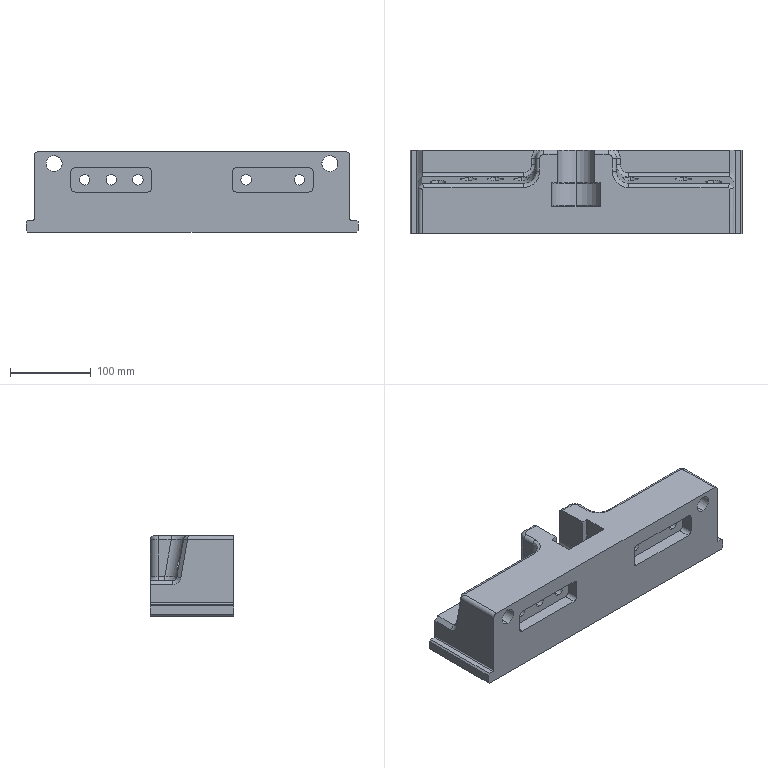Part | SolidWorks | features BaseBody 1 | 1 solid | 136 faces | box 412 x 103.35 x 100 mm | volume 3048891 mm3 | cylinder 62 | plane 59 | torus 7 | cone 4 | spline 4 | commonest cylinder face diameters 10 x22 20 x16 13 x10 2 x4 3 x2 10.5 x2